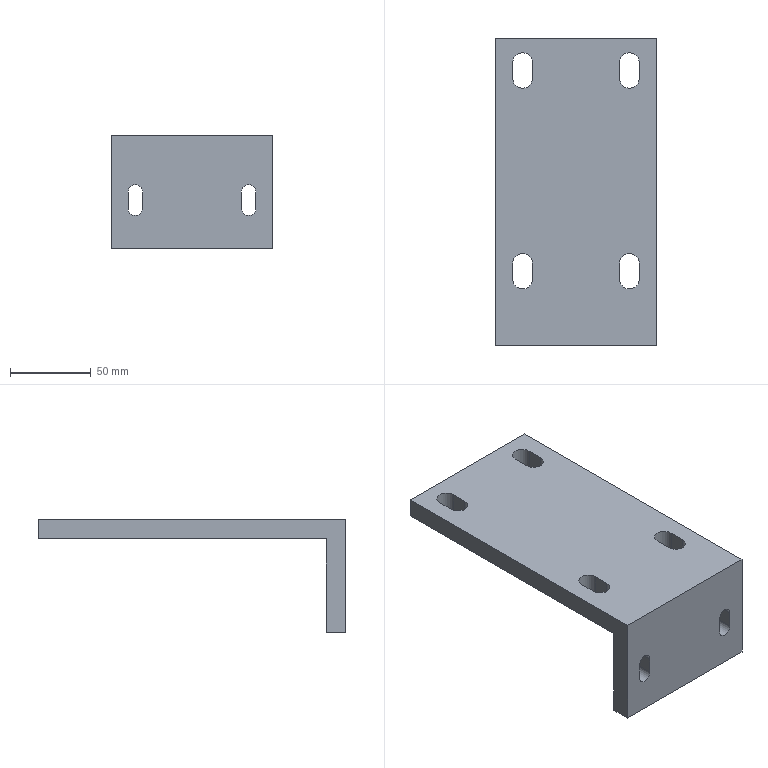Part | STEP file | PN_0002 connecting plate | 1 solid | 34 faces | box 100 x 190 x 70 mm | volume 282725 mm3 | plane 20 | cylinder 14 | commonest cylinder face diameters 12 x8 9 x6